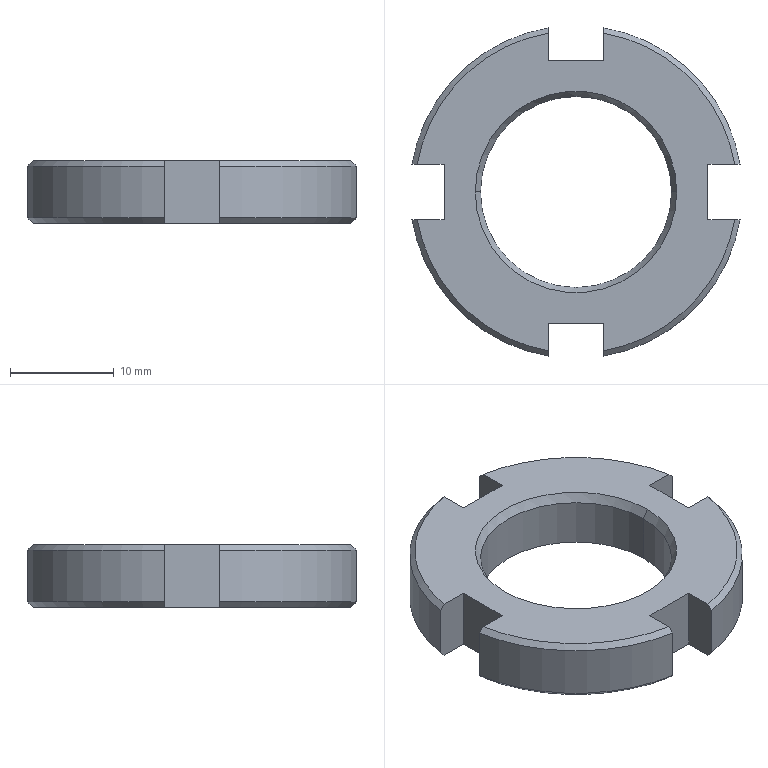Part | SolidWorks | features BaseBody 1 | 1 solid | 32 faces | box 31.558 x 31.558 x 6 mm | volume 2776 mm3 | plane 14 | cone 12 | cylinder 6 | commonest cylinder face diameters 32 x4 18.376 x2
STEP:
#1=CARTESIAN_POINT('',(-9.188,0.,-0.866));
#2=VERTEX_POINT('',#1);
#3=CARTESIAN_POINT('',(9.188,0.,-0.866));
#4=VERTEX_POINT('',#3);
#5=CARTESIAN_POINT('',(0.,0.,-0.866));
#6=DIRECTION('',(0.,0.,1.));
#7=DIRECTION('',(1.,0.,0.));
#8=AXIS2_PLACEMENT_3D('',#5,#6,#7);
#9=CIRCLE('',#8,9.188);
#10=EDGE_CURVE('',#2,#4,#9,.T.);
#11=ORIENTED_EDGE('',*,*,#10,.F.);
#12=CARTESIAN_POINT('',(-9.688,0.,0.));
#13=VERTEX_POINT('',#12);
#14=CARTESIAN_POINT('',(-9.688,0.,0.));
#15=DIRECTION('',(-0.5,0.,0.866));
#16=VECTOR('',#15,1000.);
#17=LINE('',#14,#16);
#18=EDGE_CURVE('',#2,#13,#17,.T.);
#19=ORIENTED_EDGE('',*,*,#18,.T.);
#20=CARTESIAN_POINT('',(9.688,0.,0.));
#21=VERTEX_POINT('',#20);
#22=CARTESIAN_POINT('',(0.,0.,0.));
#23=DIRECTION('',(0.,0.,-1.));
#24=DIRECTION('',(1.,0.,0.));
#25=AXIS2_PLACEMENT_3D('',#22,#23,#24);
#26=CIRCLE('',#25,9.688);
#27=EDGE_CURVE('',#21,#13,#26,.T.);
#28=ORIENTED_EDGE('',*,*,#27,.F.);
#29=CARTESIAN_POINT('',(9.688,0.,0.));
#30=DIRECTION('',(0.5,0.,0.866));
#31=VECTOR('',#30,1000.);
#32=LINE('',#29,#31);
#33=EDGE_CURVE('',#4,#21,#32,.T.);
#34=ORIENTED_EDGE('',*,*,#33,.F.);
#35=EDGE_LOOP('',(#11,#19,#28,#34));
#36=FACE_OUTER_BOUND('',#35,.T.);
#37=CARTESIAN_POINT('',(0.,0.,0.));
#38=DIRECTION('',(0.,0.,1.));
#39=DIRECTION('',(1.,0.,0.));
#40=AXIS2_PLACEMENT_3D('',#37,#38,#39);
#41=CONICAL_SURFACE('',#40,9.688,0.5236);
#42=ADVANCED_FACE('',(#36),#41,.F.);
#43=CARTESIAN_POINT('',(-9.188,0.,-5.5));
#44=VERTEX_POINT('',#43);
#45=CARTESIAN_POINT('',(9.188,0.,-5.5));
#46=VERTEX_POINT('',#45);
#47=CARTESIAN_POINT('',(0.,0.,-5.5));
#48=DIRECTION('',(0.,0.,1.));
#49=DIRECTION('',(1.,0.,0.));
#50=AXIS2_PLACEMENT_3D('',#47,#48,#49);
#51=CIRCLE('',#50,9.188);
#52=EDGE_CURVE('',#44,#46,#51,.T.);
#53=ORIENTED_EDGE('',*,*,#52,.F.);
#54=CARTESIAN_POINT('',(-9.188,0.,-6.));
#55=DIRECTION('',(0.,0.,1.));
#56=VECTOR('',#55,1000.);
#57=LINE('',#54,#56);
#58=EDGE_CURVE('',#44,#2,#57,.T.);
#59=ORIENTED_EDGE('',*,*,#58,.T.);
#60=ORIENTED_EDGE('',*,*,#10,.T.);
#61=CARTESIAN_POINT('',(9.188,0.,-6.));
#62=DIRECTION('',(0.,0.,1.));
#63=VECTOR('',#62,1000.);
#64=LINE('',#61,#63);
#65=EDGE_CURVE('',#46,#4,#64,.T.);
#66=ORIENTED_EDGE('',*,*,#65,.F.);
#67=EDGE_LOOP('',(#53,#59,#60,#66));
#68=FACE_OUTER_BOUND('',#67,.T.);
#69=CARTESIAN_POINT('',(0.,0.,-6.));
#70=DIRECTION('',(0.,0.,1.));
#71=DIRECTION('',(1.,0.,0.));
#72=AXIS2_PLACEMENT_3D('',#69,#70,#71);
#73=CYLINDRICAL_SURFACE('',#72,9.188);
#74=ADVANCED_FACE('',(#68),#73,.F.);
#75=ORIENTED_EDGE('',*,*,#52,.T.);
#76=CARTESIAN_POINT('',(10.054,0.,-6.));
#77=VERTEX_POINT('',#76);
#78=CARTESIAN_POINT('',(10.054,0.,-6.));
#79=DIRECTION('',(0.866,0.,-0.5));
#80=VECTOR('',#79,1000.);
#81=LINE('',#78,#80);
#82=EDGE_CURVE('',#46,#77,#81,.T.);
#83=ORIENTED_EDGE('',*,*,#82,.T.);
#84=CARTESIAN_POINT('',(-10.054,0.,-6.));
#85=VERTEX_POINT('',#84);
#86=CARTESIAN_POINT('',(0.,0.,-6.));
#87=DIRECTION('',(0.,0.,-1.));
#88=DIRECTION('',(-1.,0.,0.));
#89=AXIS2_PLACEMENT_3D('',#86,#87,#88);
#90=CIRCLE('',#89,10.054);
#91=EDGE_CURVE('',#77,#85,#90,.T.);
#92=ORIENTED_EDGE('',*,*,#91,.T.);
#93=CARTESIAN_POINT('',(-10.054,0.,-6.));
#94=DIRECTION('',(-0.866,0.,-0.5));
#95=VECTOR('',#94,1000.);
#96=LINE('',#93,#95);
#97=EDGE_CURVE('',#44,#85,#96,.T.);
#98=ORIENTED_EDGE('',*,*,#97,.F.);
#99=EDGE_LOOP('',(#75,#83,#92,#98));
#100=FACE_OUTER_BOUND('',#99,.T.);
#101=CARTESIAN_POINT('',(0.,0.,-6.));
#102=DIRECTION('',(0.,0.,-1.));
#103=DIRECTION('',(-1.,0.,0.));
#104=AXIS2_PLACEMENT_3D('',#101,#102,#103);
#105=CONICAL_SURFACE('',#104,10.054,1.047);
#106=ADVANCED_FACE('',(#100),#105,.F.);
#107=ORIENTED_EDGE('',*,*,#27,.T.);
#108=CARTESIAN_POINT('',(0.,0.,0.));
#109=DIRECTION('',(0.,0.,-1.));
#110=DIRECTION('',(1.,0.,0.));
#111=AXIS2_PLACEMENT_3D('',#108,#109,#110);
#112=CIRCLE('',#111,9.688);
#113=EDGE_CURVE('',#13,#21,#112,.T.);
#114=ORIENTED_EDGE('',*,*,#113,.T.);
#115=EDGE_LOOP('',(#107,#114));
#116=FACE_BOUND('',#115,.T.);
#117=CARTESIAN_POINT('',(2.65,-12.679,0.));
#118=VERTEX_POINT('',#117);
#119=CARTESIAN_POINT('',(2.65,-15.272,0.));
#120=VERTEX_POINT('',#119);
#121=CARTESIAN_POINT('',(2.65,0.,0.));
#122=DIRECTION('',(0.,-1.,0.));
#123=VECTOR('',#122,1000.);
#124=LINE('',#121,#123);
#125=EDGE_CURVE('',#118,#120,#124,.T.);
#126=ORIENTED_EDGE('',*,*,#125,.T.);
#127=CARTESIAN_POINT('',(15.272,-2.65,0.));
#128=VERTEX_POINT('',#127);
#129=CARTESIAN_POINT('',(0.,0.,0.));
#130=DIRECTION('',(0.,0.,1.));
#131=DIRECTION('',(-1.,0.,0.));
#132=AXIS2_PLACEMENT_3D('',#129,#130,#131);
#133=CIRCLE('',#132,15.5);
#134=EDGE_CURVE('',#120,#128,#133,.T.);
#135=ORIENTED_EDGE('',*,*,#134,.T.);
#136=CARTESIAN_POINT('',(12.679,-2.65,0.));
#137=VERTEX_POINT('',#136);
#138=CARTESIAN_POINT('',(0.,-2.65,0.));
#139=DIRECTION('',(-1.,0.,0.));
#140=VECTOR('',#139,1000.);
#141=LINE('',#138,#140);
#142=EDGE_CURVE('',#128,#137,#141,.T.);
#143=ORIENTED_EDGE('',*,*,#142,.T.);
#144=CARTESIAN_POINT('',(12.679,2.65,0.));
#145=VERTEX_POINT('',#144);
#146=CARTESIAN_POINT('',(12.679,0.,0.));
#147=DIRECTION('',(0.,1.,0.));
#148=VECTOR('',#147,1000.);
#149=LINE('',#146,#148);
#150=EDGE_CURVE('',#137,#145,#149,.T.);
#151=ORIENTED_EDGE('',*,*,#150,.T.);
#152=CARTESIAN_POINT('',(15.272,2.65,0.));
#153=VERTEX_POINT('',#152);
#154=CARTESIAN_POINT('',(0.,2.65,0.));
#155=DIRECTION('',(1.,0.,0.));
#156=VECTOR('',#155,1000.);
#157=LINE('',#154,#156);
#158=EDGE_CURVE('',#145,#153,#157,.T.);
#159=ORIENTED_EDGE('',*,*,#158,.T.);
#160=CARTESIAN_POINT('',(2.65,15.272,0.));
#161=VERTEX_POINT('',#160);
#162=CARTESIAN_POINT('',(0.,0.,0.));
#163=DIRECTION('',(0.,0.,1.));
#164=DIRECTION('',(-1.,0.,0.));
#165=AXIS2_PLACEMENT_3D('',#162,#163,#164);
#166=CIRCLE('',#165,15.5);
#167=EDGE_CURVE('',#153,#161,#166,.T.);
#168=ORIENTED_EDGE('',*,*,#167,.T.);
#169=CARTESIAN_POINT('',(2.65,12.679,0.));
#170=VERTEX_POINT('',#169);
#171=CARTESIAN_POINT('',(2.65,0.,0.));
#172=DIRECTION('',(0.,-1.,0.));
#173=VECTOR('',#172,1000.);
#174=LINE('',#171,#173);
#175=EDGE_CURVE('',#161,#170,#174,.T.);
#176=ORIENTED_EDGE('',*,*,#175,.T.);
#177=CARTESIAN_POINT('',(-2.65,12.679,0.));
#178=VERTEX_POINT('',#177);
#179=CARTESIAN_POINT('',(0.,12.679,0.));
#180=DIRECTION('',(-1.,0.,0.));
#181=VECTOR('',#180,1000.);
#182=LINE('',#179,#181);
#183=EDGE_CURVE('',#170,#178,#182,.T.);
#184=ORIENTED_EDGE('',*,*,#183,.T.);
#185=CARTESIAN_POINT('',(-2.65,15.272,0.));
#186=VERTEX_POINT('',#185);
#187=CARTESIAN_POINT('',(-2.65,0.,0.));
#188=DIRECTION('',(0.,1.,0.));
#189=VECTOR('',#188,1000.);
#190=LINE('',#187,#189);
#191=EDGE_CURVE('',#178,#186,#190,.T.);
#192=ORIENTED_EDGE('',*,*,#191,.T.);
#193=CARTESIAN_POINT('',(-15.272,2.65,0.));
#194=VERTEX_POINT('',#193);
#195=CARTESIAN_POINT('',(0.,0.,0.));
#196=DIRECTION('',(0.,0.,1.));
#197=DIRECTION('',(-1.,0.,0.));
#198=AXIS2_PLACEMENT_3D('',#195,#196,#197);
#199=CIRCLE('',#198,15.5);
#200=EDGE_CURVE('',#186,#194,#199,.T.);
#201=ORIENTED_EDGE('',*,*,#200,.T.);
#202=CARTESIAN_POINT('',(-12.679,2.65,0.));
#203=VERTEX_POINT('',#202);
#204=CARTESIAN_POINT('',(0.,2.65,0.));
#205=DIRECTION('',(1.,0.,0.));
#206=VECTOR('',#205,1000.);
#207=LINE('',#204,#206);
#208=EDGE_CURVE('',#194,#203,#207,.T.);
#209=ORIENTED_EDGE('',*,*,#208,.T.);
#210=CARTESIAN_POINT('',(-12.679,-2.65,0.));
#211=VERTEX_POINT('',#210);
#212=CARTESIAN_POINT('',(-12.679,0.,0.));
#213=DIRECTION('',(0.,-1.,0.));
#214=VECTOR('',#213,1000.);
#215=LINE('',#212,#214);
#216=EDGE_CURVE('',#203,#211,#215,.T.);
#217=ORIENTED_EDGE('',*,*,#216,.T.);
#218=CARTESIAN_POINT('',(-15.272,-2.65,0.));
#219=VERTEX_POINT('',#218);
#220=CARTESIAN_POINT('',(0.,-2.65,0.));
#221=DIRECTION('',(-1.,0.,0.));
#222=VECTOR('',#221,1000.);
#223=LINE('',#220,#222);
#224=EDGE_CURVE('',#211,#219,#223,.T.);
#225=ORIENTED_EDGE('',*,*,#224,.T.);
#226=CARTESIAN_POINT('',(-2.65,-15.272,0.));
#227=VERTEX_POINT('',#226);
#228=CARTESIAN_POINT('',(0.,0.,0.));
#229=DIRECTION('',(0.,0.,1.));
#230=DIRECTION('',(-1.,0.,0.));
#231=AXIS2_PLACEMENT_3D('',#228,#229,#230);
#232=CIRCLE('',#231,15.5);
#233=EDGE_CURVE('',#219,#227,#232,.T.);
#234=ORIENTED_EDGE('',*,*,#233,.T.);
#235=CARTESIAN_POINT('',(-2.65,-12.679,0.));
#236=VERTEX_POINT('',#235);
#237=CARTESIAN_POINT('',(-2.65,0.,0.));
#238=DIRECTION('',(0.,1.,0.));
#239=VECTOR('',#238,1000.);
#240=LINE('',#237,#239);
#241=EDGE_CURVE('',#227,#236,#240,.T.);
#242=ORIENTED_EDGE('',*,*,#241,.T.);
#243=CARTESIAN_POINT('',(0.,-12.679,0.));
#244=DIRECTION('',(1.,0.,0.));
#245=VECTOR('',#244,1000.);
#246=LINE('',#243,#245);
#247=EDGE_CURVE('',#236,#118,#246,.T.);
#248=ORIENTED_EDGE('',*,*,#247,.T.);
#249=EDGE_LOOP('',(#126,#135,#143,#151,#159,#168,#176,#184,#192,#201,#209,#217,#225,#234,#242,#248));
#250=FACE_OUTER_BOUND('',#249,.T.);
#251=CARTESIAN_POINT('',(0.,0.,0.));
#252=DIRECTION('',(0.,0.,1.));
#253=DIRECTION('',(1.,0.,0.));
#254=AXIS2_PLACEMENT_3D('',#251,#252,#253);
#255=PLANE('',#254);
#256=ADVANCED_FACE('',(#116,#250),#255,.T.);
#257=ORIENTED_EDGE('',*,*,#18,.F.);
#258=CARTESIAN_POINT('',(0.,0.,-0.866));
#259=DIRECTION('',(0.,0.,1.));
#260=DIRECTION('',(1.,0.,0.));
#261=AXIS2_PLACEMENT_3D('',#258,#259,#260);
#262=CIRCLE('',#261,9.188);
#263=EDGE_CURVE('',#4,#2,#262,.T.);
#264=ORIENTED_EDGE('',*,*,#263,.F.);
#265=ORIENTED_EDGE('',*,*,#33,.T.);
#266=ORIENTED_EDGE('',*,*,#113,.F.);
#267=EDGE_LOOP('',(#257,#264,#265,#266));
#268=FACE_OUTER_BOUND('',#267,.T.);
#269=CARTESIAN_POINT('',(0.,0.,0.));
#270=DIRECTION('',(0.,0.,1.));
#271=DIRECTION('',(1.,0.,0.));
#272=AXIS2_PLACEMENT_3D('',#269,#270,#271);
#273=CONICAL_SURFACE('',#272,9.688,0.5236);
#274=ADVANCED_FACE('',(#268),#273,.F.);
#275=CARTESIAN_POINT('',(2.65,-15.779,-0.5));
#276=VERTEX_POINT('',#275);
#277=CARTESIAN_POINT('',(2.65,-15.272,0.));
#278=CARTESIAN_POINT('',(2.65,-15.441,-0.1666));
#279=CARTESIAN_POINT('',(2.65,-15.61,-0.3333));
#280=CARTESIAN_POINT('',(2.65,-15.779,-0.5));
#281=B_SPLINE_CURVE_WITH_KNOTS('',3,(#277,#278,#279,#280),.UNSPECIFIED.,.F.,.F.,(4,4),(0.,0.0007122),.UNSPECIFIED.);
#282=EDGE_CURVE('',#120,#276,#281,.T.);
#283=ORIENTED_EDGE('',*,*,#282,.T.);
#284=CARTESIAN_POINT('',(15.779,-2.65,-0.5));
#285=VERTEX_POINT('',#284);
#286=CARTESIAN_POINT('',(0.,0.,-0.5));
#287=DIRECTION('',(0.,0.,1.));
#288=DIRECTION('',(-1.,0.,0.));
#289=AXIS2_PLACEMENT_3D('',#286,#287,#288);
#290=CIRCLE('',#289,16.);
#291=EDGE_CURVE('',#276,#285,#290,.T.);
#292=ORIENTED_EDGE('',*,*,#291,.T.);
#293=CARTESIAN_POINT('',(15.779,-2.65,-0.5));
#294=CARTESIAN_POINT('',(15.61,-2.65,-0.3333));
#295=CARTESIAN_POINT('',(15.441,-2.65,-0.1666));
#296=CARTESIAN_POINT('',(15.272,-2.65,0.));
#297=B_SPLINE_CURVE_WITH_KNOTS('',3,(#293,#294,#295,#296),.UNSPECIFIED.,.F.,.F.,(4,4),(0.,0.0007122),.UNSPECIFIED.);
#298=EDGE_CURVE('',#285,#128,#297,.T.);
#299=ORIENTED_EDGE('',*,*,#298,.T.);
#300=ORIENTED_EDGE('',*,*,#134,.F.);
#301=EDGE_LOOP('',(#283,#292,#299,#300));
#302=FACE_OUTER_BOUND('',#301,.T.);
#303=CARTESIAN_POINT('',(0.,0.,-0.5));
#304=DIRECTION('',(0.,0.,-1.));
#305=DIRECTION('',(-1.,0.,0.));
#306=AXIS2_PLACEMENT_3D('',#303,#304,#305);
#307=CONICAL_SURFACE('',#306,16.,0.7854);
#308=ADVANCED_FACE('',(#302),#307,.T.);
#309=CARTESIAN_POINT('',(2.65,-15.779,-5.5));
#310=VERTEX_POINT('',#309);
#311=CARTESIAN_POINT('',(2.65,-15.779,-6.));
#312=DIRECTION('',(0.,0.,-1.));
#313=VECTOR('',#312,1000.);
#314=LINE('',#311,#313);
#315=EDGE_CURVE('',#276,#310,#314,.T.);
#316=ORIENTED_EDGE('',*,*,#315,.F.);
#317=ORIENTED_EDGE('',*,*,#282,.F.);
#318=ORIENTED_EDGE('',*,*,#125,.F.);
#319=CARTESIAN_POINT('',(2.65,-12.679,-6.));
#320=VERTEX_POINT('',#319);
#321=CARTESIAN_POINT('',(2.65,-12.679,-6.));
#322=DIRECTION('',(0.,0.,1.));
#323=VECTOR('',#322,1000.);
#324=LINE('',#321,#323);
#325=EDGE_CURVE('',#320,#118,#324,.T.);
#326=ORIENTED_EDGE('',*,*,#325,.F.);
#327=CARTESIAN_POINT('',(2.65,-15.272,-6.));
#328=VERTEX_POINT('',#327);
#329=CARTESIAN_POINT('',(2.65,-15.779,-6.));
#330=DIRECTION('',(0.,1.,0.));
#331=VECTOR('',#330,1000.);
#332=LINE('',#329,#331);
#333=EDGE_CURVE('',#328,#320,#332,.T.);
#334=ORIENTED_EDGE('',*,*,#333,.F.);
#335=CARTESIAN_POINT('',(2.65,-15.779,-5.5));
#336=CARTESIAN_POINT('',(2.65,-15.61,-5.667));
#337=CARTESIAN_POINT('',(2.65,-15.441,-5.833));
#338=CARTESIAN_POINT('',(2.65,-15.272,-6.));
#339=B_SPLINE_CURVE_WITH_KNOTS('',3,(#335,#336,#337,#338),.UNSPECIFIED.,.F.,.F.,(4,4),(0.,0.0007122),.UNSPECIFIED.);
#340=EDGE_CURVE('',#310,#328,#339,.T.);
#341=ORIENTED_EDGE('',*,*,#340,.F.);
#342=EDGE_LOOP('',(#316,#317,#318,#326,#334,#341));
#343=FACE_OUTER_BOUND('',#342,.T.);
#344=CARTESIAN_POINT('',(2.65,-15.779,-6.));
#345=DIRECTION('',(1.,0.,0.));
#346=DIRECTION('',(0.,1.,0.));
#347=AXIS2_PLACEMENT_3D('',#344,#345,#346);
#348=PLANE('',#347);
#349=ADVANCED_FACE('',(#343),#348,.F.);
#350=CARTESIAN_POINT('',(-2.65,-12.679,-6.));
#351=VERTEX_POINT('',#350);
#352=CARTESIAN_POINT('',(-2.65,-12.679,-6.));
#353=DIRECTION('',(0.,0.,1.));
#354=VECTOR('',#353,1000.);
#355=LINE('',#352,#354);
#356=EDGE_CURVE('',#351,#236,#355,.T.);
#357=ORIENTED_EDGE('',*,*,#356,.F.);
#358=CARTESIAN_POINT('',(2.65,-12.679,-6.));
#359=DIRECTION('',(-1.,0.,0.));
#360=VECTOR('',#359,1000.);
#361=LINE('',#358,#360);
#362=EDGE_CURVE('',#320,#351,#361,.T.);
#363=ORIENTED_EDGE('',*,*,#362,.F.);
#364=ORIENTED_EDGE('',*,*,#325,.T.);
#365=ORIENTED_EDGE('',*,*,#247,.F.);
#366=EDGE_LOOP('',(#357,#363,#364,#365));
#367=FACE_OUTER_BOUND('',#366,.T.);
#368=CARTESIAN_POINT('',(2.65,-12.679,-6.));
#369=DIRECTION('',(0.,1.,0.));
#370=DIRECTION('',(-1.,0.,0.));
#371=AXIS2_PLACEMENT_3D('',#368,#369,#370);
#372=PLANE('',#371);
#373=ADVANCED_FACE('',(#367),#372,.F.);
#374=CARTESIAN_POINT('',(-2.65,-15.272,-6.));
#375=VERTEX_POINT('',#374);
#376=CARTESIAN_POINT('',(-2.65,-15.779,-6.));
#377=DIRECTION('',(0.,-1.,0.));
#378=VECTOR('',#377,1000.);
#379=LINE('',#376,#378);
#380=EDGE_CURVE('',#351,#375,#379,.T.);
#381=ORIENTED_EDGE('',*,*,#380,.F.);
#382=ORIENTED_EDGE('',*,*,#356,.T.);
#383=ORIENTED_EDGE('',*,*,#241,.F.);
#384=CARTESIAN_POINT('',(-2.65,-15.779,-0.5));
#385=VERTEX_POINT('',#384);
#386=CARTESIAN_POINT('',(-2.65,-15.779,-0.5));
#387=CARTESIAN_POINT('',(-2.65,-15.61,-0.3333));
#388=CARTESIAN_POINT('',(-2.65,-15.441,-0.1666));
#389=CARTESIAN_POINT('',(-2.65,-15.272,0.));
#390=B_SPLINE_CURVE_WITH_KNOTS('',3,(#386,#387,#388,#389),.UNSPECIFIED.,.F.,.F.,(4,4),(0.,0.0007122),.UNSPECIFIED.);
#391=EDGE_CURVE('',#385,#227,#390,.T.);
#392=ORIENTED_EDGE('',*,*,#391,.F.);
#393=CARTESIAN_POINT('',(-2.65,-15.779,-5.5));
#394=VERTEX_POINT('',#393);
#395=CARTESIAN_POINT('',(-2.65,-15.779,-6.));
#396=DIRECTION('',(0.,0.,1.));
#397=VECTOR('',#396,1000.);
#398=LINE('',#395,#397);
#399=EDGE_CURVE('',#394,#385,#398,.T.);
#400=ORIENTED_EDGE('',*,*,#399,.F.);
#401=CARTESIAN_POINT('',(-2.65,-15.272,-6.));
#402=CARTESIAN_POINT('',(-2.65,-15.441,-5.833));
#403=CARTESIAN_POINT('',(-2.65,-15.61,-5.667));
#404=CARTESIAN_POINT('',(-2.65,-15.779,-5.5));
#405=B_SPLINE_CURVE_WITH_KNOTS('',3,(#401,#402,#403,#404),.UNSPECIFIED.,.F.,.F.,(4,4),(0.,0.0007122),.UNSPECIFIED.);
#406=EDGE_CURVE('',#375,#394,#405,.T.);
#407=ORIENTED_EDGE('',*,*,#406,.F.);
#408=EDGE_LOOP('',(#381,#382,#383,#392,#400,#407));
#409=FACE_OUTER_BOUND('',#408,.T.);
#410=CARTESIAN_POINT('',(-2.65,-15.779,-6.));
#411=DIRECTION('',(-1.,0.,0.));
#412=DIRECTION('',(0.,-1.,0.));
#413=AXIS2_PLACEMENT_3D('',#410,#411,#412);
#414=PLANE('',#413);
#415=ADVANCED_FACE('',(#409),#414,.F.);
#416=CARTESIAN_POINT('',(-15.779,-2.65,-0.5));
#417=VERTEX_POINT('',#416);
#418=CARTESIAN_POINT('',(-15.272,-2.65,0.));
#419=CARTESIAN_POINT('',(-15.441,-2.65,-0.1666));
#420=CARTESIAN_POINT('',(-15.61,-2.65,-0.3333));
#421=CARTESIAN_POINT('',(-15.779,-2.65,-0.5));
#422=B_SPLINE_CURVE_WITH_KNOTS('',3,(#418,#419,#420,#421),.UNSPECIFIED.,.F.,.F.,(4,4),(0.,0.0007122),.UNSPECIFIED.);
#423=EDGE_CURVE('',#219,#417,#422,.T.);
#424=ORIENTED_EDGE('',*,*,#423,.T.);
#425=CARTESIAN_POINT('',(0.,0.,-0.5));
#426=DIRECTION('',(0.,0.,1.));
#427=DIRECTION('',(-1.,0.,0.));
#428=AXIS2_PLACEMENT_3D('',#425,#426,#427);
#429=CIRCLE('',#428,16.);
#430=EDGE_CURVE('',#417,#385,#429,.T.);
#431=ORIENTED_EDGE('',*,*,#430,.T.);
#432=ORIENTED_EDGE('',*,*,#391,.T.);
#433=ORIENTED_EDGE('',*,*,#233,.F.);
#434=EDGE_LOOP('',(#424,#431,#432,#433));
#435=FACE_OUTER_BOUND('',#434,.T.);
#436=CARTESIAN_POINT('',(0.,0.,-0.5));
#437=DIRECTION('',(0.,0.,-1.));
#438=DIRECTION('',(-1.,0.,0.));
#439=AXIS2_PLACEMENT_3D('',#436,#437,#438);
#440=CONICAL_SURFACE('',#439,16.,0.7854);
#441=ADVANCED_FACE('',(#435),#440,.T.);
#442=CARTESIAN_POINT('',(-15.779,-2.65,-5.5));
#443=VERTEX_POINT('',#442);
#444=CARTESIAN_POINT('',(-15.779,-2.65,-6.));
#445=DIRECTION('',(0.,0.,-1.));
#446=VECTOR('',#445,1000.);
#447=LINE('',#444,#446);
#448=EDGE_CURVE('',#417,#443,#447,.T.);
#449=ORIENTED_EDGE('',*,*,#448,.F.);
#450=ORIENTED_EDGE('',*,*,#423,.F.);
#451=ORIENTED_EDGE('',*,*,#224,.F.);
#452=CARTESIAN_POINT('',(-12.679,-2.65,-6.));
#453=VERTEX_POINT('',#452);
#454=CARTESIAN_POINT('',(-12.679,-2.65,-6.));
#455=DIRECTION('',(0.,0.,1.));
#456=VECTOR('',#455,1000.);
#457=LINE('',#454,#456);
#458=EDGE_CURVE('',#453,#211,#457,.T.);
#459=ORIENTED_EDGE('',*,*,#458,.F.);
#460=CARTESIAN_POINT('',(-15.272,-2.65,-6.));
#461=VERTEX_POINT('',#460);
#462=CARTESIAN_POINT('',(-15.779,-2.65,-6.));
#463=DIRECTION('',(1.,0.,0.));
#464=VECTOR('',#463,1000.);
#465=LINE('',#462,#464);
#466=EDGE_CURVE('',#461,#453,#465,.T.);
#467=ORIENTED_EDGE('',*,*,#466,.F.);
#468=CARTESIAN_POINT('',(-15.779,-2.65,-5.5));
#469=CARTESIAN_POINT('',(-15.61,-2.65,-5.667));
#470=CARTESIAN_POINT('',(-15.441,-2.65,-5.833));
#471=CARTESIAN_POINT('',(-15.272,-2.65,-6.));
#472=B_SPLINE_CURVE_WITH_KNOTS('',3,(#468,#469,#470,#471),.UNSPECIFIED.,.F.,.F.,(4,4),(0.,0.0007122),.UNSPECIFIED.);
#473=EDGE_CURVE('',#443,#461,#472,.T.);
#474=ORIENTED_EDGE('',*,*,#473,.F.);
#475=EDGE_LOOP('',(#449,#450,#451,#459,#467,#474));
#476=FACE_OUTER_BOUND('',#475,.T.);
#477=CARTESIAN_POINT('',(-15.779,-2.65,-6.));
#478=DIRECTION('',(0.,-1.,0.));
#479=DIRECTION('',(1.,0.,0.));
#480=AXIS2_PLACEMENT_3D('',#477,#478,#479);
#481=PLANE('',#480);
#482=ADVANCED_FACE('',(#476),#481,.F.);
#483=CARTESIAN_POINT('',(-12.679,2.65,-6.));
#484=VERTEX_POINT('',#483);
#485=CARTESIAN_POINT('',(-12.679,2.65,-6.));
#486=DIRECTION('',(0.,0.,1.));
#487=VECTOR('',#486,1000.);
#488=LINE('',#485,#487);
#489=EDGE_CURVE('',#484,#203,#488,.T.);
#490=ORIENTED_EDGE('',*,*,#489,.F.);
#491=CARTESIAN_POINT('',(-12.679,-2.65,-6.));
#492=DIRECTION('',(0.,1.,0.));
#493=VECTOR('',#492,1000.);
#494=LINE('',#491,#493);
#495=EDGE_CURVE('',#453,#484,#494,.T.);
#496=ORIENTED_EDGE('',*,*,#495,.F.);
#497=ORIENTED_EDGE('',*,*,#458,.T.);
#498=ORIENTED_EDGE('',*,*,#216,.F.);
#499=EDGE_LOOP('',(#490,#496,#497,#498));
#500=FACE_OUTER_BOUND('',#499,.T.);
#501=CARTESIAN_POINT('',(-12.679,-2.65,-6.));
#502=DIRECTION('',(1.,0.,0.));
#503=DIRECTION('',(0.,1.,0.));
#504=AXIS2_PLACEMENT_3D('',#501,#502,#503);
#505=PLANE('',#504);
#506=ADVANCED_FACE('',(#500),#505,.F.);
#507=CARTESIAN_POINT('',(-15.272,2.65,-6.));
#508=VERTEX_POINT('',#507);
#509=CARTESIAN_POINT('',(-15.779,2.65,-6.));
#510=DIRECTION('',(-1.,0.,0.));
#511=VECTOR('',#510,1000.);
#512=LINE('',#509,#511);
#513=EDGE_CURVE('',#484,#508,#512,.T.);
#514=ORIENTED_EDGE('',*,*,#513,.F.);
#515=ORIENTED_EDGE('',*,*,#489,.T.);
#516=ORIENTED_EDGE('',*,*,#208,.F.);
#517=CARTESIAN_POINT('',(-15.779,2.65,-0.5));
#518=VERTEX_POINT('',#517);
#519=CARTESIAN_POINT('',(-15.779,2.65,-0.5));
#520=CARTESIAN_POINT('',(-15.61,2.65,-0.3333));
#521=CARTESIAN_POINT('',(-15.441,2.65,-0.1666));
#522=CARTESIAN_POINT('',(-15.272,2.65,0.));
#523=B_SPLINE_CURVE_WITH_KNOTS('',3,(#519,#520,#521,#522),.UNSPECIFIED.,.F.,.F.,(4,4),(0.,0.0007122),.UNSPECIFIED.);
#524=EDGE_CURVE('',#518,#194,#523,.T.);
#525=ORIENTED_EDGE('',*,*,#524,.F.);
#526=CARTESIAN_POINT('',(-15.779,2.65,-5.5));
#527=VERTEX_POINT('',#526);
#528=CARTESIAN_POINT('',(-15.779,2.65,-6.));
#529=DIRECTION('',(0.,0.,1.));
#530=VECTOR('',#529,1000.);
#531=LINE('',#528,#530);
#532=EDGE_CURVE('',#527,#518,#531,.T.);
#533=ORIENTED_EDGE('',*,*,#532,.F.);
#534=CARTESIAN_POINT('',(-15.272,2.65,-6.));
#535=CARTESIAN_POINT('',(-15.441,2.65,-5.833));
#536=CARTESIAN_POINT('',(-15.61,2.65,-5.667));
#537=CARTESIAN_POINT('',(-15.779,2.65,-5.5));
#538=B_SPLINE_CURVE_WITH_KNOTS('',3,(#534,#535,#536,#537),.UNSPECIFIED.,.F.,.F.,(4,4),(0.,0.0007122),.UNSPECIFIED.);
#539=EDGE_CURVE('',#508,#527,#538,.T.);
#540=ORIENTED_EDGE('',*,*,#539,.F.);
#541=EDGE_LOOP('',(#514,#515,#516,#525,#533,#540));
#542=FACE_OUTER_BOUND('',#541,.T.);
#543=CARTESIAN_POINT('',(-15.779,2.65,-6.));
#544=DIRECTION('',(0.,1.,0.));
#545=DIRECTION('',(-1.,0.,0.));
#546=AXIS2_PLACEMENT_3D('',#543,#544,#545);
#547=PLANE('',#546);
#548=ADVANCED_FACE('',(#542),#547,.F.);
#549=CARTESIAN_POINT('',(-2.65,15.779,-0.5));
#550=VERTEX_POINT('',#549);
#551=CARTESIAN_POINT('',(-2.65,15.272,0.));
#552=CARTESIAN_POINT('',(-2.65,15.441,-0.1666));
#553=CARTESIAN_POINT('',(-2.65,15.61,-0.3333));
#554=CARTESIAN_POINT('',(-2.65,15.779,-0.5));
#555=B_SPLINE_CURVE_WITH_KNOTS('',3,(#551,#552,#553,#554),.UNSPECIFIED.,.F.,.F.,(4,4),(0.,0.0007122),.UNSPECIFIED.);
#556=EDGE_CURVE('',#186,#550,#555,.T.);
#557=ORIENTED_EDGE('',*,*,#556,.T.);
#558=CARTESIAN_POINT('',(0.,0.,-0.5));
#559=DIRECTION('',(0.,0.,1.));
#560=DIRECTION('',(-1.,0.,0.));
#561=AXIS2_PLACEMENT_3D('',#558,#559,#560);
#562=CIRCLE('',#561,16.);
#563=EDGE_CURVE('',#550,#518,#562,.T.);
#564=ORIENTED_EDGE('',*,*,#563,.T.);
#565=ORIENTED_EDGE('',*,*,#524,.T.);
#566=ORIENTED_EDGE('',*,*,#200,.F.);
#567=EDGE_LOOP('',(#557,#564,#565,#566));
#568=FACE_OUTER_BOUND('',#567,.T.);
#569=CARTESIAN_POINT('',(0.,0.,-0.5));
#570=DIRECTION('',(0.,0.,-1.));
#571=DIRECTION('',(-1.,0.,0.));
#572=AXIS2_PLACEMENT_3D('',#569,#570,#571);
#573=CONICAL_SURFACE('',#572,16.,0.7854);
#574=ADVANCED_FACE('',(#568),#573,.T.);
#575=CARTESIAN_POINT('',(-2.65,15.779,-5.5));
#576=VERTEX_POINT('',#575);
#577=CARTESIAN_POINT('',(-2.65,15.779,-6.));
#578=DIRECTION('',(0.,0.,-1.));
#579=VECTOR('',#578,1000.);
#580=LINE('',#577,#579);
#581=EDGE_CURVE('',#550,#576,#580,.T.);
#582=ORIENTED_EDGE('',*,*,#581,.F.);
#583=ORIENTED_EDGE('',*,*,#556,.F.);
#584=ORIENTED_EDGE('',*,*,#191,.F.);
#585=CARTESIAN_POINT('',(-2.65,12.679,-6.));
#586=VERTEX_POINT('',#585);
#587=CARTESIAN_POINT('',(-2.65,12.679,-6.));
#588=DIRECTION('',(0.,0.,1.));
#589=VECTOR('',#588,1000.);
#590=LINE('',#587,#589);
#591=EDGE_CURVE('',#586,#178,#590,.T.);
#592=ORIENTED_EDGE('',*,*,#591,.F.);
#593=CARTESIAN_POINT('',(-2.65,15.272,-6.));
#594=VERTEX_POINT('',#593);
#595=CARTESIAN_POINT('',(-2.65,15.779,-6.));
#596=DIRECTION('',(0.,-1.,0.));
#597=VECTOR('',#596,1000.);
#598=LINE('',#595,#597);
#599=EDGE_CURVE('',#594,#586,#598,.T.);
#600=ORIENTED_EDGE('',*,*,#599,.F.);
#601=CARTESIAN_POINT('',(-2.65,15.779,-5.5));
#602=CARTESIAN_POINT('',(-2.65,15.61,-5.667));
#603=CARTESIAN_POINT('',(-2.65,15.441,-5.833));
#604=CARTESIAN_POINT('',(-2.65,15.272,-6.));
#605=B_SPLINE_CURVE_WITH_KNOTS('',3,(#601,#602,#603,#604),.UNSPECIFIED.,.F.,.F.,(4,4),(0.,0.0007122),.UNSPECIFIED.);
#606=EDGE_CURVE('',#576,#594,#605,.T.);
#607=ORIENTED_EDGE('',*,*,#606,.F.);
#608=EDGE_LOOP('',(#582,#583,#584,#592,#600,#607));
#609=FACE_OUTER_BOUND('',#608,.T.);
#610=CARTESIAN_POINT('',(-2.65,15.779,-6.));
#611=DIRECTION('',(-1.,0.,0.));
#612=DIRECTION('',(0.,-1.,0.));
#613=AXIS2_PLACEMENT_3D('',#610,#611,#612);
#614=PLANE('',#613);
#615=ADVANCED_FACE('',(#609),#614,.F.);
#616=CARTESIAN_POINT('',(2.65,12.679,-6.));
#617=VERTEX_POINT('',#616);
#618=CARTESIAN_POINT('',(2.65,12.679,-6.));
#619=DIRECTION('',(0.,0.,1.));
#620=VECTOR('',#619,1000.);
#621=LINE('',#618,#620);
#622=EDGE_CURVE('',#617,#170,#621,.T.);
#623=ORIENTED_EDGE('',*,*,#622,.F.);
#624=CARTESIAN_POINT('',(-2.65,12.679,-6.));
#625=DIRECTION('',(1.,0.,0.));
#626=VECTOR('',#625,1000.);
#627=LINE('',#624,#626);
#628=EDGE_CURVE('',#586,#617,#627,.T.);
#629=ORIENTED_EDGE('',*,*,#628,.F.);
#630=ORIENTED_EDGE('',*,*,#591,.T.);
#631=ORIENTED_EDGE('',*,*,#183,.F.);
#632=EDGE_LOOP('',(#623,#629,#630,#631));
#633=FACE_OUTER_BOUND('',#632,.T.);
#634=CARTESIAN_POINT('',(-2.65,12.679,-6.));
#635=DIRECTION('',(0.,-1.,0.));
#636=DIRECTION('',(0.,0.,-1.));
#637=AXIS2_PLACEMENT_3D('',#634,#635,#636);
#638=PLANE('',#637);
#639=ADVANCED_FACE('',(#633),#638,.F.);
#640=CARTESIAN_POINT('',(2.65,15.272,-6.));
#641=VERTEX_POINT('',#640);
#642=CARTESIAN_POINT('',(2.65,15.779,-6.));
#643=DIRECTION('',(0.,1.,0.));
#644=VECTOR('',#643,1000.);
#645=LINE('',#642,#644);
#646=EDGE_CURVE('',#617,#641,#645,.T.);
#647=ORIENTED_EDGE('',*,*,#646,.F.);
#648=ORIENTED_EDGE('',*,*,#622,.T.);
#649=ORIENTED_EDGE('',*,*,#175,.F.);
#650=CARTESIAN_POINT('',(2.65,15.779,-0.5));
#651=VERTEX_POINT('',#650);
#652=CARTESIAN_POINT('',(2.65,15.779,-0.5));
#653=CARTESIAN_POINT('',(2.65,15.61,-0.3333));
#654=CARTESIAN_POINT('',(2.65,15.441,-0.1666));
#655=CARTESIAN_POINT('',(2.65,15.272,0.));
#656=B_SPLINE_CURVE_WITH_KNOTS('',3,(#652,#653,#654,#655),.UNSPECIFIED.,.F.,.F.,(4,4),(0.,0.0007122),.UNSPECIFIED.);
#657=EDGE_CURVE('',#651,#161,#656,.T.);
#658=ORIENTED_EDGE('',*,*,#657,.F.);
#659=CARTESIAN_POINT('',(2.65,15.779,-5.5));
#660=VERTEX_POINT('',#659);
#661=CARTESIAN_POINT('',(2.65,15.779,-6.));
#662=DIRECTION('',(0.,0.,1.));
#663=VECTOR('',#662,1000.);
#664=LINE('',#661,#663);
#665=EDGE_CURVE('',#660,#651,#664,.T.);
#666=ORIENTED_EDGE('',*,*,#665,.F.);
#667=CARTESIAN_POINT('',(2.65,15.272,-6.));
#668=CARTESIAN_POINT('',(2.65,15.441,-5.833));
#669=CARTESIAN_POINT('',(2.65,15.61,-5.667));
#670=CARTESIAN_POINT('',(2.65,15.779,-5.5));
#671=B_SPLINE_CURVE_WITH_KNOTS('',3,(#667,#668,#669,#670),.UNSPECIFIED.,.F.,.F.,(4,4),(0.,0.0007122),.UNSPECIFIED.);
#672=EDGE_CURVE('',#641,#660,#671,.T.);
#673=ORIENTED_EDGE('',*,*,#672,.F.);
#674=EDGE_LOOP('',(#647,#648,#649,#658,#666,#673));
#675=FACE_OUTER_BOUND('',#674,.T.);
#676=CARTESIAN_POINT('',(2.65,15.779,-6.));
#677=DIRECTION('',(1.,0.,0.));
#678=DIRECTION('',(0.,1.,0.));
#679=AXIS2_PLACEMENT_3D('',#676,#677,#678);
#680=PLANE('',#679);
#681=ADVANCED_FACE('',(#675),#680,.F.);
#682=ORIENTED_EDGE('',*,*,#657,.T.);
#683=ORIENTED_EDGE('',*,*,#167,.F.);
#684=CARTESIAN_POINT('',(15.779,2.65,-0.5));
#685=VERTEX_POINT('',#684);
#686=CARTESIAN_POINT('',(15.272,2.65,0.));
#687=CARTESIAN_POINT('',(15.441,2.65,-0.1666));
#688=CARTESIAN_POINT('',(15.61,2.65,-0.3333));
#689=CARTESIAN_POINT('',(15.779,2.65,-0.5));
#690=B_SPLINE_CURVE_WITH_KNOTS('',3,(#686,#687,#688,#689),.UNSPECIFIED.,.F.,.F.,(4,4),(0.,0.0007122),.UNSPECIFIED.);
#691=EDGE_CURVE('',#153,#685,#690,.T.);
#692=ORIENTED_EDGE('',*,*,#691,.T.);
#693=CARTESIAN_POINT('',(0.,0.,-0.5));
#694=DIRECTION('',(0.,0.,1.));
#695=DIRECTION('',(-1.,0.,0.));
#696=AXIS2_PLACEMENT_3D('',#693,#694,#695);
#697=CIRCLE('',#696,16.);
#698=EDGE_CURVE('',#685,#651,#697,.T.);
#699=ORIENTED_EDGE('',*,*,#698,.T.);
#700=EDGE_LOOP('',(#682,#683,#692,#699));
#701=FACE_OUTER_BOUND('',#700,.T.);
#702=CARTESIAN_POINT('',(0.,0.,-0.5));
#703=DIRECTION('',(0.,0.,-1.));
#704=DIRECTION('',(-1.,0.,0.));
#705=AXIS2_PLACEMENT_3D('',#702,#703,#704);
#706=CONICAL_SURFACE('',#705,16.,0.7854);
#707=ADVANCED_FACE('',(#701),#706,.T.);
#708=CARTESIAN_POINT('',(15.779,2.65,-5.5));
#709=VERTEX_POINT('',#708);
#710=CARTESIAN_POINT('',(15.779,2.65,-6.));
#711=DIRECTION('',(0.,0.,-1.));
#712=VECTOR('',#711,1000.);
#713=LINE('',#710,#712);
#714=EDGE_CURVE('',#685,#709,#713,.T.);
#715=ORIENTED_EDGE('',*,*,#714,.F.);
#716=ORIENTED_EDGE('',*,*,#691,.F.);
#717=ORIENTED_EDGE('',*,*,#158,.F.);
#718=CARTESIAN_POINT('',(12.679,2.65,-6.));
#719=VERTEX_POINT('',#718);
#720=CARTESIAN_POINT('',(12.679,2.65,-6.));
#721=DIRECTION('',(0.,0.,1.));
#722=VECTOR('',#721,1000.);
#723=LINE('',#720,#722);
#724=EDGE_CURVE('',#719,#145,#723,.T.);
#725=ORIENTED_EDGE('',*,*,#724,.F.);
#726=CARTESIAN_POINT('',(15.272,2.65,-6.));
#727=VERTEX_POINT('',#726);
#728=CARTESIAN_POINT('',(15.779,2.65,-6.));
#729=DIRECTION('',(-1.,0.,0.));
#730=VECTOR('',#729,1000.);
#731=LINE('',#728,#730);
#732=EDGE_CURVE('',#727,#719,#731,.T.);
#733=ORIENTED_EDGE('',*,*,#732,.F.);
#734=CARTESIAN_POINT('',(15.779,2.65,-5.5));
#735=CARTESIAN_POINT('',(15.61,2.65,-5.667));
#736=CARTESIAN_POINT('',(15.441,2.65,-5.833));
#737=CARTESIAN_POINT('',(15.272,2.65,-6.));
#738=B_SPLINE_CURVE_WITH_KNOTS('',3,(#734,#735,#736,#737),.UNSPECIFIED.,.F.,.F.,(4,4),(0.,0.0007122),.UNSPECIFIED.);
#739=EDGE_CURVE('',#709,#727,#738,.T.);
#740=ORIENTED_EDGE('',*,*,#739,.F.);
#741=EDGE_LOOP('',(#715,#716,#717,#725,#733,#740));
#742=FACE_OUTER_BOUND('',#741,.T.);
#743=CARTESIAN_POINT('',(15.779,2.65,-6.));
#744=DIRECTION('',(0.,1.,0.));
#745=DIRECTION('',(-1.,0.,0.));
#746=AXIS2_PLACEMENT_3D('',#743,#744,#745);
#747=PLANE('',#746);
#748=ADVANCED_FACE('',(#742),#747,.F.);
#749=CARTESIAN_POINT('',(12.679,-2.65,-6.));
#750=VERTEX_POINT('',#749);
#751=CARTESIAN_POINT('',(12.679,-2.65,-6.));
#752=DIRECTION('',(0.,0.,1.));
#753=VECTOR('',#752,1000.);
#754=LINE('',#751,#753);
#755=EDGE_CURVE('',#750,#137,#754,.T.);
#756=ORIENTED_EDGE('',*,*,#755,.F.);
#757=CARTESIAN_POINT('',(12.679,2.65,-6.));
#758=DIRECTION('',(0.,-1.,0.));
#759=VECTOR('',#758,1000.);
#760=LINE('',#757,#759);
#761=EDGE_CURVE('',#719,#750,#760,.T.);
#762=ORIENTED_EDGE('',*,*,#761,.F.);
#763=ORIENTED_EDGE('',*,*,#724,.T.);
#764=ORIENTED_EDGE('',*,*,#150,.F.);
#765=EDGE_LOOP('',(#756,#762,#763,#764));
#766=FACE_OUTER_BOUND('',#765,.T.);
#767=CARTESIAN_POINT('',(12.679,2.65,-6.));
#768=DIRECTION('',(-1.,0.,0.));
#769=DIRECTION('',(0.,-1.,0.));
#770=AXIS2_PLACEMENT_3D('',#767,#768,#769);
#771=PLANE('',#770);
#772=ADVANCED_FACE('',(#766),#771,.F.);
#773=CARTESIAN_POINT('',(15.272,-2.65,-6.));
#774=VERTEX_POINT('',#773);
#775=CARTESIAN_POINT('',(15.779,-2.65,-6.));
#776=DIRECTION('',(1.,0.,0.));
#777=VECTOR('',#776,1000.);
#778=LINE('',#775,#777);
#779=EDGE_CURVE('',#750,#774,#778,.T.);
#780=ORIENTED_EDGE('',*,*,#779,.F.);
#781=ORIENTED_EDGE('',*,*,#755,.T.);
#782=ORIENTED_EDGE('',*,*,#142,.F.);
#783=ORIENTED_EDGE('',*,*,#298,.F.);
#784=CARTESIAN_POINT('',(15.779,-2.65,-5.5));
#785=VERTEX_POINT('',#784);
#786=CARTESIAN_POINT('',(15.779,-2.65,-6.));
#787=DIRECTION('',(0.,0.,1.));
#788=VECTOR('',#787,1000.);
#789=LINE('',#786,#788);
#790=EDGE_CURVE('',#785,#285,#789,.T.);
#791=ORIENTED_EDGE('',*,*,#790,.F.);
#792=CARTESIAN_POINT('',(15.272,-2.65,-6.));
#793=CARTESIAN_POINT('',(15.441,-2.65,-5.833));
#794=CARTESIAN_POINT('',(15.61,-2.65,-5.667));
#795=CARTESIAN_POINT('',(15.779,-2.65,-5.5));
#796=B_SPLINE_CURVE_WITH_KNOTS('',3,(#792,#793,#794,#795),.UNSPECIFIED.,.F.,.F.,(4,4),(0.,0.0007122),.UNSPECIFIED.);
#797=EDGE_CURVE('',#774,#785,#796,.T.);
#798=ORIENTED_EDGE('',*,*,#797,.F.);
#799=EDGE_LOOP('',(#780,#781,#782,#783,#791,#798));
#800=FACE_OUTER_BOUND('',#799,.T.);
#801=CARTESIAN_POINT('',(15.779,-2.65,-6.));
#802=DIRECTION('',(0.,-1.,0.));
#803=DIRECTION('',(1.,0.,0.));
#804=AXIS2_PLACEMENT_3D('',#801,#802,#803);
#805=PLANE('',#804);
#806=ADVANCED_FACE('',(#800),#805,.F.);
#807=ORIENTED_EDGE('',*,*,#58,.F.);
#808=CARTESIAN_POINT('',(0.,0.,-5.5));
#809=DIRECTION('',(0.,0.,1.));
#810=DIRECTION('',(1.,0.,0.));
#811=AXIS2_PLACEMENT_3D('',#808,#809,#810);
#812=CIRCLE('',#811,9.188);
#813=EDGE_CURVE('',#46,#44,#812,.T.);
#814=ORIENTED_EDGE('',*,*,#813,.F.);
#815=ORIENTED_EDGE('',*,*,#65,.T.);
#816=ORIENTED_EDGE('',*,*,#263,.T.);
#817=EDGE_LOOP('',(#807,#814,#815,#816));
#818=FACE_OUTER_BOUND('',#817,.T.);
#819=CARTESIAN_POINT('',(0.,0.,-6.));
#820=DIRECTION('',(0.,0.,1.));
#821=DIRECTION('',(1.,0.,0.));
#822=AXIS2_PLACEMENT_3D('',#819,#820,#821);
#823=CYLINDRICAL_SURFACE('',#822,9.188);
#824=ADVANCED_FACE('',(#818),#823,.F.);
#825=ORIENTED_EDGE('',*,*,#315,.T.);
#826=CARTESIAN_POINT('',(0.,0.,-5.5));
#827=DIRECTION('',(0.,0.,1.));
#828=DIRECTION('',(1.,0.,0.));
#829=AXIS2_PLACEMENT_3D('',#826,#827,#828);
#830=CIRCLE('',#829,16.);
#831=EDGE_CURVE('',#310,#785,#830,.T.);
#832=ORIENTED_EDGE('',*,*,#831,.T.);
#833=ORIENTED_EDGE('',*,*,#790,.T.);
#834=ORIENTED_EDGE('',*,*,#291,.F.);
#835=EDGE_LOOP('',(#825,#832,#833,#834));
#836=FACE_OUTER_BOUND('',#835,.T.);
#837=CARTESIAN_POINT('',(0.,0.,-6.));
#838=DIRECTION('',(0.,0.,1.));
#839=DIRECTION('',(1.,0.,0.));
#840=AXIS2_PLACEMENT_3D('',#837,#838,#839);
#841=CYLINDRICAL_SURFACE('',#840,16.);
#842=ADVANCED_FACE('',(#836),#841,.T.);
#843=ORIENTED_EDGE('',*,*,#779,.T.);
#844=CARTESIAN_POINT('',(0.,0.,-6.));
#845=DIRECTION('',(0.,0.,1.));
#846=DIRECTION('',(1.,0.,0.));
#847=AXIS2_PLACEMENT_3D('',#844,#845,#846);
#848=CIRCLE('',#847,15.5);
#849=EDGE_CURVE('',#328,#774,#848,.T.);
#850=ORIENTED_EDGE('',*,*,#849,.F.);
#851=ORIENTED_EDGE('',*,*,#333,.T.);
#852=ORIENTED_EDGE('',*,*,#362,.T.);
#853=ORIENTED_EDGE('',*,*,#380,.T.);
#854=CARTESIAN_POINT('',(0.,0.,-6.));
#855=DIRECTION('',(0.,0.,1.));
#856=DIRECTION('',(0.,-1.,0.));
#857=AXIS2_PLACEMENT_3D('',#854,#855,#856);
#858=CIRCLE('',#857,15.5);
#859=EDGE_CURVE('',#461,#375,#858,.T.);
#860=ORIENTED_EDGE('',*,*,#859,.F.);
#861=ORIENTED_EDGE('',*,*,#466,.T.);
#862=ORIENTED_EDGE('',*,*,#495,.T.);
#863=ORIENTED_EDGE('',*,*,#513,.T.);
#864=CARTESIAN_POINT('',(0.,0.,-6.));
#865=DIRECTION('',(0.,0.,1.));
#866=DIRECTION('',(1.,0.,0.));
#867=AXIS2_PLACEMENT_3D('',#864,#865,#866);
#868=CIRCLE('',#867,15.5);
#869=EDGE_CURVE('',#594,#508,#868,.T.);
#870=ORIENTED_EDGE('',*,*,#869,.F.);
#871=ORIENTED_EDGE('',*,*,#599,.T.);
#872=ORIENTED_EDGE('',*,*,#628,.T.);
#873=ORIENTED_EDGE('',*,*,#646,.T.);
#874=CARTESIAN_POINT('',(0.,0.,-6.));
#875=DIRECTION('',(0.,0.,1.));
#876=DIRECTION('',(1.,0.,0.));
#877=AXIS2_PLACEMENT_3D('',#874,#875,#876);
#878=CIRCLE('',#877,15.5);
#879=EDGE_CURVE('',#727,#641,#878,.T.);
#880=ORIENTED_EDGE('',*,*,#879,.F.);
#881=ORIENTED_EDGE('',*,*,#732,.T.);
#882=ORIENTED_EDGE('',*,*,#761,.T.);
#883=EDGE_LOOP('',(#843,#850,#851,#852,#853,#860,#861,#862,#863,#870,#871,#872,#873,#880,#881,#882));
#884=FACE_OUTER_BOUND('',#883,.T.);
#885=CARTESIAN_POINT('',(0.,0.,-6.));
#886=DIRECTION('',(0.,0.,-1.));
#887=DIRECTION('',(-1.,0.,0.));
#888=AXIS2_PLACEMENT_3D('',#885,#886,#887);
#889=CIRCLE('',#888,10.054);
#890=EDGE_CURVE('',#85,#77,#889,.T.);
#891=ORIENTED_EDGE('',*,*,#890,.F.);
#892=ORIENTED_EDGE('',*,*,#91,.F.);
#893=EDGE_LOOP('',(#891,#892));
#894=FACE_BOUND('',#893,.T.);
#895=CARTESIAN_POINT('',(0.,0.,-6.));
#896=DIRECTION('',(0.,0.,1.));
#897=DIRECTION('',(1.,0.,0.));
#898=AXIS2_PLACEMENT_3D('',#895,#896,#897);
#899=PLANE('',#898);
#900=ADVANCED_FACE('',(#884,#894),#899,.F.);
#901=ORIENTED_EDGE('',*,*,#448,.T.);
#902=CARTESIAN_POINT('',(0.,0.,-5.5));
#903=DIRECTION('',(0.,0.,1.));
#904=DIRECTION('',(1.,0.,0.));
#905=AXIS2_PLACEMENT_3D('',#902,#903,#904);
#906=CIRCLE('',#905,16.);
#907=EDGE_CURVE('',#443,#394,#906,.T.);
#908=ORIENTED_EDGE('',*,*,#907,.T.);
#909=ORIENTED_EDGE('',*,*,#399,.T.);
#910=ORIENTED_EDGE('',*,*,#430,.F.);
#911=EDGE_LOOP('',(#901,#908,#909,#910));
#912=FACE_OUTER_BOUND('',#911,.T.);
#913=CARTESIAN_POINT('',(0.,0.,-6.));
#914=DIRECTION('',(0.,0.,1.));
#915=DIRECTION('',(1.,0.,0.));
#916=AXIS2_PLACEMENT_3D('',#913,#914,#915);
#917=CYLINDRICAL_SURFACE('',#916,16.);
#918=ADVANCED_FACE('',(#912),#917,.T.);
#919=ORIENTED_EDGE('',*,*,#581,.T.);
#920=CARTESIAN_POINT('',(0.,0.,-5.5));
#921=DIRECTION('',(0.,0.,1.));
#922=DIRECTION('',(1.,0.,0.));
#923=AXIS2_PLACEMENT_3D('',#920,#921,#922);
#924=CIRCLE('',#923,16.);
#925=EDGE_CURVE('',#576,#527,#924,.T.);
#926=ORIENTED_EDGE('',*,*,#925,.T.);
#927=ORIENTED_EDGE('',*,*,#532,.T.);
#928=ORIENTED_EDGE('',*,*,#563,.F.);
#929=EDGE_LOOP('',(#919,#926,#927,#928));
#930=FACE_OUTER_BOUND('',#929,.T.);
#931=CARTESIAN_POINT('',(0.,0.,-6.));
#932=DIRECTION('',(0.,0.,1.));
#933=DIRECTION('',(1.,0.,0.));
#934=AXIS2_PLACEMENT_3D('',#931,#932,#933);
#935=CYLINDRICAL_SURFACE('',#934,16.);
#936=ADVANCED_FACE('',(#930),#935,.T.);
#937=ORIENTED_EDGE('',*,*,#665,.T.);
#938=ORIENTED_EDGE('',*,*,#698,.F.);
#939=ORIENTED_EDGE('',*,*,#714,.T.);
#940=CARTESIAN_POINT('',(0.,0.,-5.5));
#941=DIRECTION('',(0.,0.,1.));
#942=DIRECTION('',(1.,0.,0.));
#943=AXIS2_PLACEMENT_3D('',#940,#941,#942);
#944=CIRCLE('',#943,16.);
#945=EDGE_CURVE('',#709,#660,#944,.T.);
#946=ORIENTED_EDGE('',*,*,#945,.T.);
#947=EDGE_LOOP('',(#937,#938,#939,#946));
#948=FACE_OUTER_BOUND('',#947,.T.);
#949=CARTESIAN_POINT('',(0.,0.,-6.));
#950=DIRECTION('',(0.,0.,1.));
#951=DIRECTION('',(1.,0.,0.));
#952=AXIS2_PLACEMENT_3D('',#949,#950,#951);
#953=CYLINDRICAL_SURFACE('',#952,16.);
#954=ADVANCED_FACE('',(#948),#953,.T.);
#955=ORIENTED_EDGE('',*,*,#82,.F.);
#956=ORIENTED_EDGE('',*,*,#813,.T.);
#957=ORIENTED_EDGE('',*,*,#97,.T.);
#958=ORIENTED_EDGE('',*,*,#890,.T.);
#959=EDGE_LOOP('',(#955,#956,#957,#958));
#960=FACE_OUTER_BOUND('',#959,.T.);
#961=CARTESIAN_POINT('',(0.,0.,-6.));
#962=DIRECTION('',(0.,0.,-1.));
#963=DIRECTION('',(-1.,0.,0.));
#964=AXIS2_PLACEMENT_3D('',#961,#962,#963);
#965=CONICAL_SURFACE('',#964,10.054,1.047);
#966=ADVANCED_FACE('',(#960),#965,.F.);
#967=ORIENTED_EDGE('',*,*,#340,.T.);
#968=ORIENTED_EDGE('',*,*,#849,.T.);
#969=ORIENTED_EDGE('',*,*,#797,.T.);
#970=ORIENTED_EDGE('',*,*,#831,.F.);
#971=EDGE_LOOP('',(#967,#968,#969,#970));
#972=FACE_OUTER_BOUND('',#971,.T.);
#973=CARTESIAN_POINT('',(0.,0.,-5.5));
#974=DIRECTION('',(0.,0.,1.));
#975=DIRECTION('',(1.,0.,0.));
#976=AXIS2_PLACEMENT_3D('',#973,#974,#975);
#977=CONICAL_SURFACE('',#976,16.,0.7854);
#978=ADVANCED_FACE('',(#972),#977,.T.);
#979=ORIENTED_EDGE('',*,*,#473,.T.);
#980=ORIENTED_EDGE('',*,*,#859,.T.);
#981=ORIENTED_EDGE('',*,*,#406,.T.);
#982=ORIENTED_EDGE('',*,*,#907,.F.);
#983=EDGE_LOOP('',(#979,#980,#981,#982));
#984=FACE_OUTER_BOUND('',#983,.T.);
#985=CARTESIAN_POINT('',(0.,0.,-5.5));
#986=DIRECTION('',(0.,0.,1.));
#987=DIRECTION('',(0.,-1.,0.));
#988=AXIS2_PLACEMENT_3D('',#985,#986,#987);
#989=CONICAL_SURFACE('',#988,16.,0.7854);
#990=ADVANCED_FACE('',(#984),#989,.T.);
#991=ORIENTED_EDGE('',*,*,#606,.T.);
#992=ORIENTED_EDGE('',*,*,#869,.T.);
#993=ORIENTED_EDGE('',*,*,#539,.T.);
#994=ORIENTED_EDGE('',*,*,#925,.F.);
#995=EDGE_LOOP('',(#991,#992,#993,#994));
#996=FACE_OUTER_BOUND('',#995,.T.);
#997=CARTESIAN_POINT('',(0.,0.,-5.5));
#998=DIRECTION('',(0.,0.,1.));
#999=DIRECTION('',(1.,0.,0.));
#1000=AXIS2_PLACEMENT_3D('',#997,#998,#999);
#1001=CONICAL_SURFACE('',#1000,16.,0.7854);
#1002=ADVANCED_FACE('',(#996),#1001,.T.);
#1003=ORIENTED_EDGE('',*,*,#672,.T.);
#1004=ORIENTED_EDGE('',*,*,#945,.F.);
#1005=ORIENTED_EDGE('',*,*,#739,.T.);
#1006=ORIENTED_EDGE('',*,*,#879,.T.);
#1007=EDGE_LOOP('',(#1003,#1004,#1005,#1006));
#1008=FACE_OUTER_BOUND('',#1007,.T.);
#1009=CARTESIAN_POINT('',(0.,0.,-5.5));
#1010=DIRECTION('',(0.,0.,1.));
#1011=DIRECTION('',(1.,0.,0.));
#1012=AXIS2_PLACEMENT_3D('',#1009,#1010,#1011);
#1013=CONICAL_SURFACE('',#1012,16.,0.7854);
#1014=ADVANCED_FACE('',(#1008),#1013,.T.);
#1015=CLOSED_SHELL('',(#42,#74,#106,#256,#274,#308,#349,#373,#415,#441,#482,#506,#548,#574,#615,#639,#681,#707,#748,#772,#806,#824,#842,#900,#918,#936,#954,#966,#978,#990,#1002,#1014));
#1016=MANIFOLD_SOLID_BREP('',#1015);
#1017=CARTESIAN_POINT('',(0.,0.,0.));
#1018=DIRECTION('',(0.,0.,1.));
#1019=DIRECTION('',(1.,0.,0.));
#1020=AXIS2_PLACEMENT_3D('',#1017,#1018,#1019);
#1021=(LENGTH_UNIT()NAMED_UNIT(*)SI_UNIT(.MILLI.,.METRE.));
#1022=UNCERTAINTY_MEASURE_WITH_UNIT(LENGTH_MEASURE(0.00001),#1021,'','');
#1023=(NAMED_UNIT(*)PLANE_ANGLE_UNIT()SI_UNIT($,.RADIAN.));
#1024=(NAMED_UNIT(*)SI_UNIT($,.STERADIAN.)SOLID_ANGLE_UNIT());
#1025=(GEOMETRIC_REPRESENTATION_CONTEXT(3)GLOBAL_UNCERTAINTY_ASSIGNED_CONTEXT((#1022))GLOBAL_UNIT_ASSIGNED_CONTEXT((#1021,#1023,#1024))REPRESENTATION_CONTEXT('',''));
#1026=ADVANCED_BREP_SHAPE_REPRESENTATION('',(#1016,#1020),#1025);